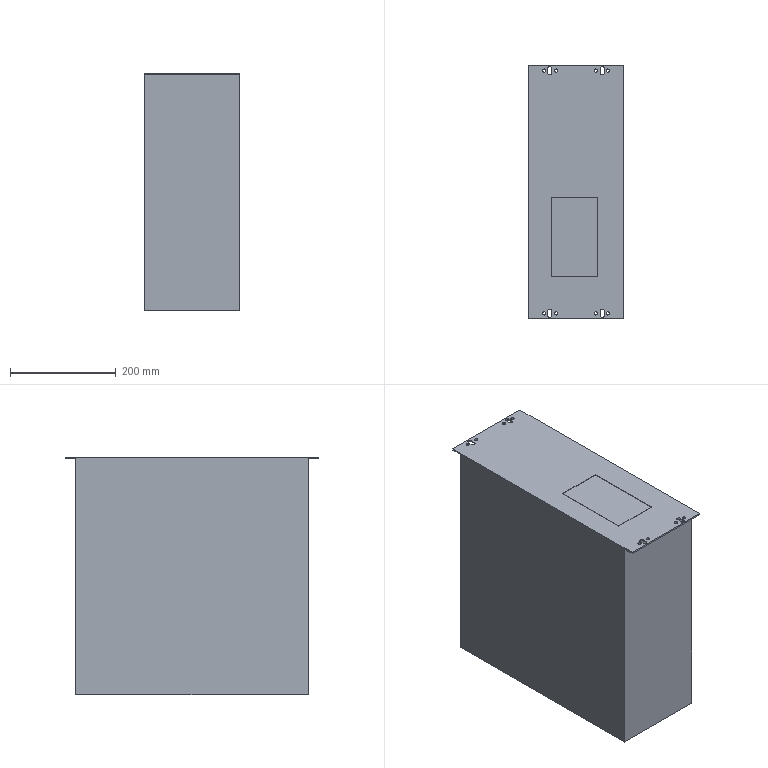Part | STEP file | Industrial PC | 1 solid | 47 faces | box 180 x 480 x 450 mm | volume 35646453 mm3 | cylinder 24 | plane 23 | commonest cylinder face diameters 6 x16 8 x8